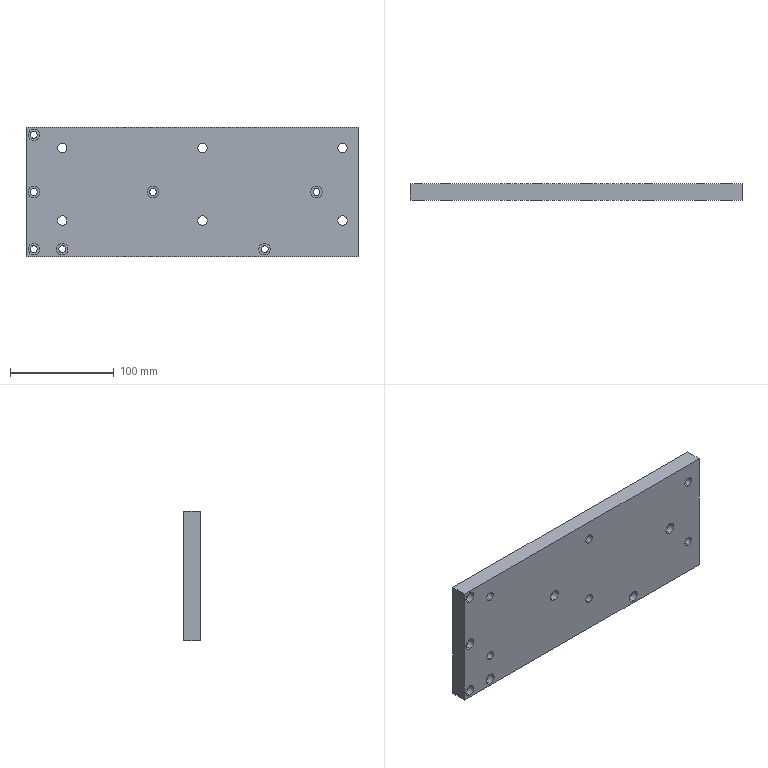Part | STEP file | 0244_208_Plate | 1 solid | 53 faces | box 320 x 16 x 125 mm | volume 627294 mm3 | cylinder 40 | plane 13 | commonest cylinder face diameters 6.6 x14 11 x14 9 x12